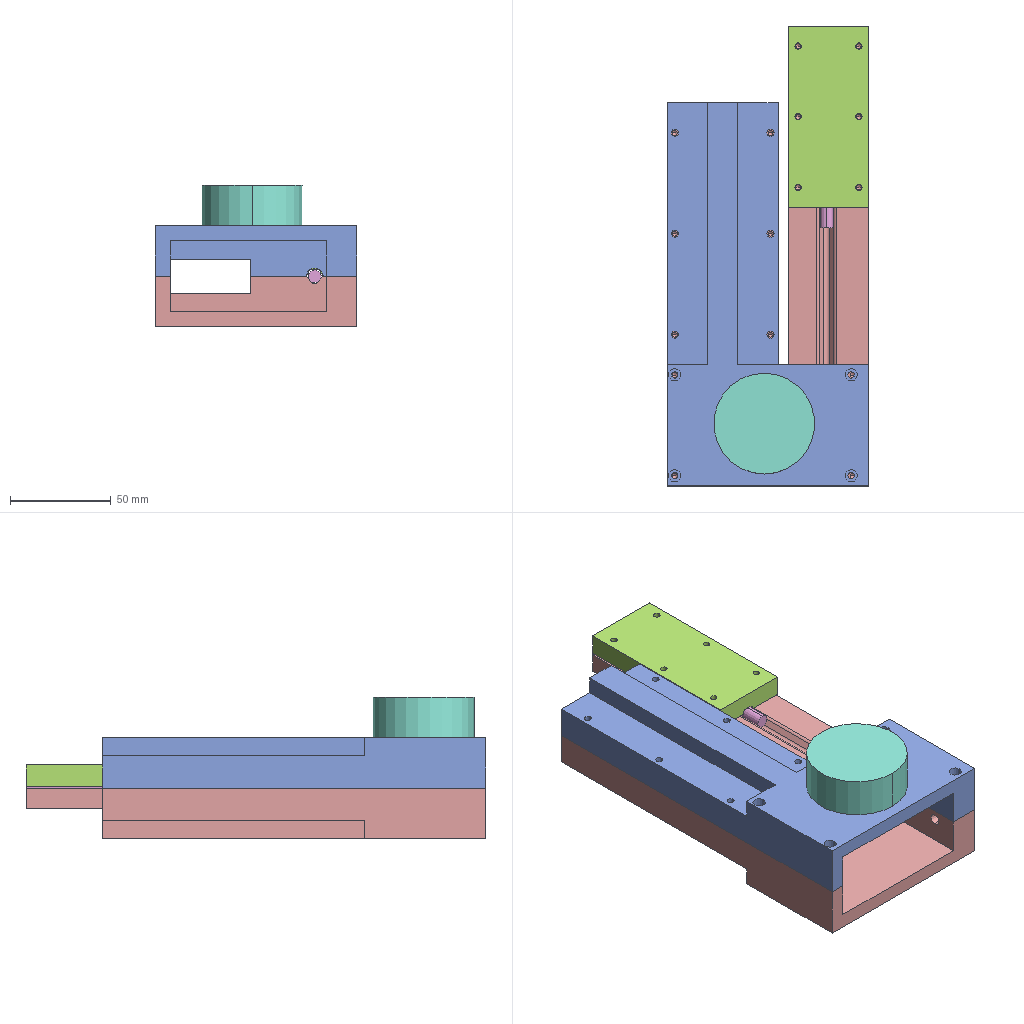Assembly | SolidWorks | 5 different items | 5 placed | box 100 x 228 x 70 mm
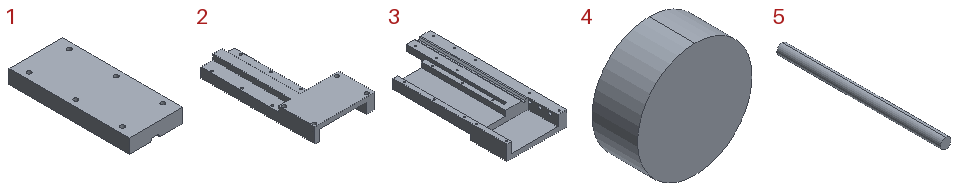Parts list (item | quantity | size | volume | features):
1 | x1 | 40 x 90 x 10.5 mm | 36117 mm3 | features ICE 5, Extrusion 1, Fillet 1, MoveFace 1
2 | x1 | 100 x 190 x 25 mm | 163793 mm3 | features ICE 11, Extrusion 1, Fillet 1, MoveFace 1
3 | x1 | 100 x 228 x 25 mm | 243999 mm3 | features ICE 8, HoleWzd 3, Extrusion 1, Fillet 1, MoveFace 1
4 | x1 | 50 x 20 x 50 mm | 39270 mm3 | features Extrusion 1
5 | x1 | 6.35 x 100 x 6.35 mm | 3167 mm3 | features Extrusion 1
Mates (type | each side: item.copy, entity, surface, feature):
Coincident | 3.1 face plane Boss-Extrude3 | 2.1 face plane Cut-Extrude1
Concentric | 3.1 face cylinder M3 Tapped Hole1 | 2.1 face cylinder Cut-Extrude3 | 2 times
Tangent | 3.1 face plane Boss-Extrude3 | 5.1 face cylinder Boss-Extrude1 | 2 times
Coincident | 3.1 face plane Boss-Extrude3 | 5.1 face plane Boss-Extrude1
Tangent | 1.1 face plane Boss-Extrude3 | 5.1 face cylinder Boss-Extrude1
Parallel | 3.1 face plane Boss-Extrude3 | 1.1 face plane Boss-Extrude3
Concentric | 3.1 face cylinder M3 Tapped Hole1 | 1.1 edge
Concentric | 3.1 face cylinder M3 Tapped Hole1 | 1.1 face cylinder Cut-Extrude3
Coincident | 2.1 face plane Boss-Extrude1 | 4.1 face plane Boss-Extrude1